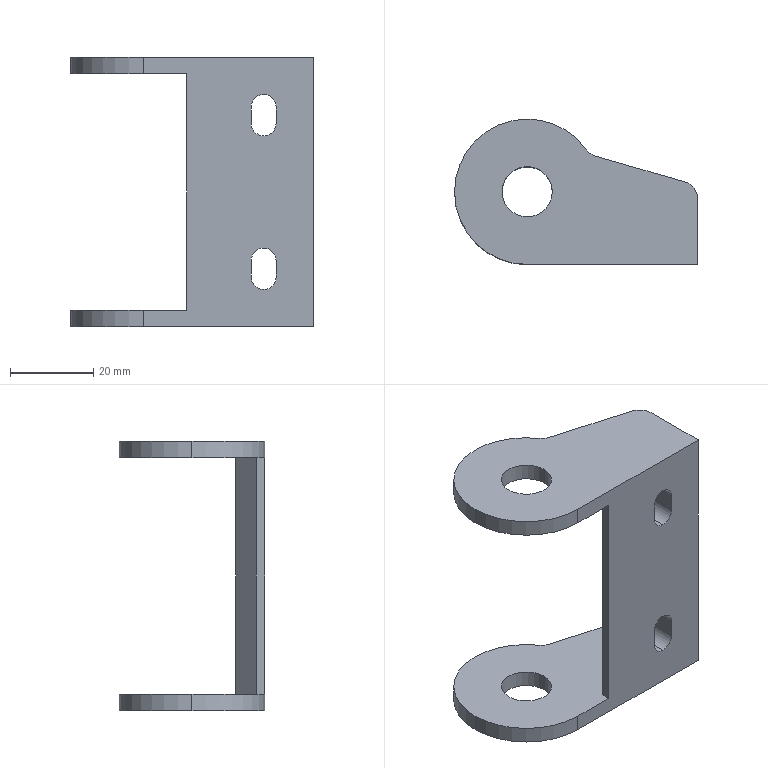Part | SolidWorks | features BaseBody 1 | 1 solid | 33 faces | box 58.5 x 35 x 65 mm | volume 22276 mm3 | cylinder 18 | plane 15 | commonest cylinder face diameters 6 x6 8 x4 12.1 x4 35 x4
STEP:
#1=CARTESIAN_POINT('',(-6.05,17.5,-28.5));
#2=VERTEX_POINT('',#1);
#3=CARTESIAN_POINT('',(6.05,17.5,-28.5));
#4=VERTEX_POINT('',#3);
#5=CARTESIAN_POINT('',(0.,17.5,-28.5));
#6=DIRECTION('',(0.,0.,1.));
#7=DIRECTION('',(1.,0.,0.));
#8=AXIS2_PLACEMENT_3D('',#5,#6,#7);
#9=CIRCLE('',#8,6.05);
#10=EDGE_CURVE('',#2,#4,#9,.T.);
#11=ORIENTED_EDGE('',*,*,#10,.T.);
#12=CARTESIAN_POINT('',(6.05,17.5,-32.5));
#13=VERTEX_POINT('',#12);
#14=CARTESIAN_POINT('',(6.05,17.5,32.5));
#15=DIRECTION('',(0.,0.,-1.));
#16=VECTOR('',#15,1000.);
#17=LINE('',#14,#16);
#18=EDGE_CURVE('',#4,#13,#17,.T.);
#19=ORIENTED_EDGE('',*,*,#18,.T.);
#20=CARTESIAN_POINT('',(-6.05,17.5,-32.5));
#21=VERTEX_POINT('',#20);
#22=CARTESIAN_POINT('',(0.,17.5,-32.5));
#23=DIRECTION('',(0.,0.,1.));
#24=DIRECTION('',(1.,0.,0.));
#25=AXIS2_PLACEMENT_3D('',#22,#23,#24);
#26=CIRCLE('',#25,6.05);
#27=EDGE_CURVE('',#21,#13,#26,.T.);
#28=ORIENTED_EDGE('',*,*,#27,.F.);
#29=CARTESIAN_POINT('',(-6.05,17.5,32.5));
#30=DIRECTION('',(0.,0.,-1.));
#31=VECTOR('',#30,1000.);
#32=LINE('',#29,#31);
#33=EDGE_CURVE('',#2,#21,#32,.T.);
#34=ORIENTED_EDGE('',*,*,#33,.F.);
#35=EDGE_LOOP('',(#11,#19,#28,#34));
#36=FACE_OUTER_BOUND('',#35,.T.);
#37=CARTESIAN_POINT('',(0.,17.5,32.5));
#38=DIRECTION('',(0.,0.,-1.));
#39=DIRECTION('',(-1.,0.,0.));
#40=AXIS2_PLACEMENT_3D('',#37,#38,#39);
#41=CYLINDRICAL_SURFACE('',#40,6.05);
#42=ADVANCED_FACE('',(#36),#41,.F.);
#43=CARTESIAN_POINT('',(-6.05,17.5,32.5));
#44=VERTEX_POINT('',#43);
#45=CARTESIAN_POINT('',(6.05,17.5,32.5));
#46=VERTEX_POINT('',#45);
#47=CARTESIAN_POINT('',(0.,17.5,32.5));
#48=DIRECTION('',(0.,0.,1.));
#49=DIRECTION('',(1.,0.,0.));
#50=AXIS2_PLACEMENT_3D('',#47,#48,#49);
#51=CIRCLE('',#50,6.05);
#52=EDGE_CURVE('',#44,#46,#51,.T.);
#53=ORIENTED_EDGE('',*,*,#52,.T.);
#54=CARTESIAN_POINT('',(6.05,17.5,28.5));
#55=VERTEX_POINT('',#54);
#56=CARTESIAN_POINT('',(6.05,17.5,32.5));
#57=DIRECTION('',(0.,0.,-1.));
#58=VECTOR('',#57,1000.);
#59=LINE('',#56,#58);
#60=EDGE_CURVE('',#46,#55,#59,.T.);
#61=ORIENTED_EDGE('',*,*,#60,.T.);
#62=CARTESIAN_POINT('',(-6.05,17.5,28.5));
#63=VERTEX_POINT('',#62);
#64=CARTESIAN_POINT('',(0.,17.5,28.5));
#65=DIRECTION('',(0.,0.,1.));
#66=DIRECTION('',(1.,0.,0.));
#67=AXIS2_PLACEMENT_3D('',#64,#65,#66);
#68=CIRCLE('',#67,6.05);
#69=EDGE_CURVE('',#63,#55,#68,.T.);
#70=ORIENTED_EDGE('',*,*,#69,.F.);
#71=CARTESIAN_POINT('',(-6.05,17.5,32.5));
#72=DIRECTION('',(0.,0.,-1.));
#73=VECTOR('',#72,1000.);
#74=LINE('',#71,#73);
#75=EDGE_CURVE('',#44,#63,#74,.T.);
#76=ORIENTED_EDGE('',*,*,#75,.F.);
#77=EDGE_LOOP('',(#53,#61,#70,#76));
#78=FACE_OUTER_BOUND('',#77,.T.);
#79=CARTESIAN_POINT('',(0.,17.5,32.5));
#80=DIRECTION('',(0.,0.,-1.));
#81=DIRECTION('',(-1.,0.,0.));
#82=AXIS2_PLACEMENT_3D('',#79,#80,#81);
#83=CYLINDRICAL_SURFACE('',#82,6.05);
#84=ADVANCED_FACE('',(#78),#83,.F.);
#85=CARTESIAN_POINT('',(29.,7.,13.5));
#86=VERTEX_POINT('',#85);
#87=CARTESIAN_POINT('',(32.,7.,16.5));
#88=VERTEX_POINT('',#87);
#89=CARTESIAN_POINT('',(29.,7.,16.5));
#90=DIRECTION('',(0.,-1.,0.));
#91=DIRECTION('',(-1.,0.,0.));
#92=AXIS2_PLACEMENT_3D('',#89,#90,#91);
#93=CIRCLE('',#92,3.);
#94=EDGE_CURVE('',#86,#88,#93,.T.);
#95=ORIENTED_EDGE('',*,*,#94,.F.);
#96=CARTESIAN_POINT('',(29.,0.,13.5));
#97=VERTEX_POINT('',#96);
#98=CARTESIAN_POINT('',(29.,10.,13.5));
#99=DIRECTION('',(0.,-1.,0.));
#100=VECTOR('',#99,1000.);
#101=LINE('',#98,#100);
#102=EDGE_CURVE('',#86,#97,#101,.T.);
#103=ORIENTED_EDGE('',*,*,#102,.T.);
#104=CARTESIAN_POINT('',(32.,0.,16.5));
#105=VERTEX_POINT('',#104);
#106=CARTESIAN_POINT('',(29.,0.,16.5));
#107=DIRECTION('',(0.,1.,0.));
#108=DIRECTION('',(1.,0.,0.));
#109=AXIS2_PLACEMENT_3D('',#106,#107,#108);
#110=CIRCLE('',#109,3.);
#111=EDGE_CURVE('',#105,#97,#110,.T.);
#112=ORIENTED_EDGE('',*,*,#111,.F.);
#113=CARTESIAN_POINT('',(32.,7.,16.5));
#114=DIRECTION('',(0.,-1.,0.));
#115=VECTOR('',#114,1000.);
#116=LINE('',#113,#115);
#117=EDGE_CURVE('',#88,#105,#116,.T.);
#118=ORIENTED_EDGE('',*,*,#117,.F.);
#119=EDGE_LOOP('',(#95,#103,#112,#118));
#120=FACE_OUTER_BOUND('',#119,.T.);
#121=CARTESIAN_POINT('',(29.,10.,16.5));
#122=DIRECTION('',(0.,-1.,0.));
#123=DIRECTION('',(0.,0.,-1.));
#124=AXIS2_PLACEMENT_3D('',#121,#122,#123);
#125=CYLINDRICAL_SURFACE('',#124,3.);
#126=ADVANCED_FACE('',(#120),#125,.F.);
#127=CARTESIAN_POINT('',(29.,7.,-23.5));
#128=VERTEX_POINT('',#127);
#129=CARTESIAN_POINT('',(32.,7.,-20.5));
#130=VERTEX_POINT('',#129);
#131=CARTESIAN_POINT('',(29.,7.,-20.5));
#132=DIRECTION('',(0.,-1.,0.));
#133=DIRECTION('',(-1.,0.,0.));
#134=AXIS2_PLACEMENT_3D('',#131,#132,#133);
#135=CIRCLE('',#134,3.);
#136=EDGE_CURVE('',#128,#130,#135,.T.);
#137=ORIENTED_EDGE('',*,*,#136,.F.);
#138=CARTESIAN_POINT('',(29.,0.,-23.5));
#139=VERTEX_POINT('',#138);
#140=CARTESIAN_POINT('',(29.,10.,-23.5));
#141=DIRECTION('',(0.,-1.,0.));
#142=VECTOR('',#141,1000.);
#143=LINE('',#140,#142);
#144=EDGE_CURVE('',#128,#139,#143,.T.);
#145=ORIENTED_EDGE('',*,*,#144,.T.);
#146=CARTESIAN_POINT('',(32.,0.,-20.5));
#147=VERTEX_POINT('',#146);
#148=CARTESIAN_POINT('',(29.,0.,-20.5));
#149=DIRECTION('',(0.,1.,0.));
#150=DIRECTION('',(1.,0.,0.));
#151=AXIS2_PLACEMENT_3D('',#148,#149,#150);
#152=CIRCLE('',#151,3.);
#153=EDGE_CURVE('',#147,#139,#152,.T.);
#154=ORIENTED_EDGE('',*,*,#153,.F.);
#155=CARTESIAN_POINT('',(32.,7.,-20.5));
#156=DIRECTION('',(0.,-1.,0.));
#157=VECTOR('',#156,1000.);
#158=LINE('',#155,#157);
#159=EDGE_CURVE('',#130,#147,#158,.T.);
#160=ORIENTED_EDGE('',*,*,#159,.F.);
#161=EDGE_LOOP('',(#137,#145,#154,#160));
#162=FACE_OUTER_BOUND('',#161,.T.);
#163=CARTESIAN_POINT('',(29.,10.,-20.5));
#164=DIRECTION('',(0.,-1.,0.));
#165=DIRECTION('',(0.,0.,-1.));
#166=AXIS2_PLACEMENT_3D('',#163,#164,#165);
#167=CYLINDRICAL_SURFACE('',#166,3.);
#168=ADVANCED_FACE('',(#162),#167,.F.);
#169=CARTESIAN_POINT('',(-17.5,17.5,-28.5));
#170=VERTEX_POINT('',#169);
#171=CARTESIAN_POINT('',(0.,0.,-28.5));
#172=VERTEX_POINT('',#171);
#173=CARTESIAN_POINT('',(0.,17.5,-28.5));
#174=DIRECTION('',(0.,0.,1.));
#175=DIRECTION('',(0.8159,0.5783,0.));
#176=AXIS2_PLACEMENT_3D('',#173,#174,#175);
#177=CIRCLE('',#176,17.5);
#178=EDGE_CURVE('',#170,#172,#177,.T.);
#179=ORIENTED_EDGE('',*,*,#178,.F.);
#180=CARTESIAN_POINT('',(-17.5,17.5,-32.5));
#181=VERTEX_POINT('',#180);
#182=CARTESIAN_POINT('',(-17.5,17.5,32.5));
#183=DIRECTION('',(0.,0.,-1.));
#184=VECTOR('',#183,1000.);
#185=LINE('',#182,#184);
#186=EDGE_CURVE('',#170,#181,#185,.T.);
#187=ORIENTED_EDGE('',*,*,#186,.T.);
#188=CARTESIAN_POINT('',(0.,0.,-32.5));
#189=VERTEX_POINT('',#188);
#190=CARTESIAN_POINT('',(0.,17.5,-32.5));
#191=DIRECTION('',(0.,0.,1.));
#192=DIRECTION('',(0.8159,0.5783,0.));
#193=AXIS2_PLACEMENT_3D('',#190,#191,#192);
#194=CIRCLE('',#193,17.5);
#195=EDGE_CURVE('',#181,#189,#194,.T.);
#196=ORIENTED_EDGE('',*,*,#195,.T.);
#197=CARTESIAN_POINT('',(0.,0.,-28.5));
#198=DIRECTION('',(0.,0.,-1.));
#199=VECTOR('',#198,1000.);
#200=LINE('',#197,#199);
#201=EDGE_CURVE('',#172,#189,#200,.T.);
#202=ORIENTED_EDGE('',*,*,#201,.F.);
#203=EDGE_LOOP('',(#179,#187,#196,#202));
#204=FACE_OUTER_BOUND('',#203,.T.);
#205=CARTESIAN_POINT('',(0.,17.5,32.5));
#206=DIRECTION('',(0.,0.,-1.));
#207=DIRECTION('',(-1.,0.,0.));
#208=AXIS2_PLACEMENT_3D('',#205,#206,#207);
#209=CYLINDRICAL_SURFACE('',#208,17.5);
#210=ADVANCED_FACE('',(#204),#209,.T.);
#211=CARTESIAN_POINT('',(-17.5,17.5,32.5));
#212=VERTEX_POINT('',#211);
#213=CARTESIAN_POINT('',(0.,0.,32.5));
#214=VERTEX_POINT('',#213);
#215=CARTESIAN_POINT('',(0.,17.5,32.5));
#216=DIRECTION('',(0.,0.,1.));
#217=DIRECTION('',(0.8159,0.5783,0.));
#218=AXIS2_PLACEMENT_3D('',#215,#216,#217);
#219=CIRCLE('',#218,17.5);
#220=EDGE_CURVE('',#212,#214,#219,.T.);
#221=ORIENTED_EDGE('',*,*,#220,.F.);
#222=CARTESIAN_POINT('',(-17.5,17.5,28.5));
#223=VERTEX_POINT('',#222);
#224=CARTESIAN_POINT('',(-17.5,17.5,32.5));
#225=DIRECTION('',(0.,0.,-1.));
#226=VECTOR('',#225,1000.);
#227=LINE('',#224,#226);
#228=EDGE_CURVE('',#212,#223,#227,.T.);
#229=ORIENTED_EDGE('',*,*,#228,.T.);
#230=CARTESIAN_POINT('',(0.,0.,28.5));
#231=VERTEX_POINT('',#230);
#232=CARTESIAN_POINT('',(0.,17.5,28.5));
#233=DIRECTION('',(0.,0.,1.));
#234=DIRECTION('',(0.8159,0.5783,0.));
#235=AXIS2_PLACEMENT_3D('',#232,#233,#234);
#236=CIRCLE('',#235,17.5);
#237=EDGE_CURVE('',#223,#231,#236,.T.);
#238=ORIENTED_EDGE('',*,*,#237,.T.);
#239=CARTESIAN_POINT('',(0.,0.,32.5));
#240=DIRECTION('',(0.,0.,-1.));
#241=VECTOR('',#240,1000.);
#242=LINE('',#239,#241);
#243=EDGE_CURVE('',#214,#231,#242,.T.);
#244=ORIENTED_EDGE('',*,*,#243,.F.);
#245=EDGE_LOOP('',(#221,#229,#238,#244));
#246=FACE_OUTER_BOUND('',#245,.T.);
#247=CARTESIAN_POINT('',(0.,17.5,32.5));
#248=DIRECTION('',(0.,0.,-1.));
#249=DIRECTION('',(-1.,0.,0.));
#250=AXIS2_PLACEMENT_3D('',#247,#248,#249);
#251=CYLINDRICAL_SURFACE('',#250,17.5);
#252=ADVANCED_FACE('',(#246),#251,.T.);
#253=ORIENTED_EDGE('',*,*,#243,.T.);
#254=CARTESIAN_POINT('',(10.5,0.,28.5));
#255=VERTEX_POINT('',#254);
#256=CARTESIAN_POINT('',(0.,0.,28.5));
#257=DIRECTION('',(1.,0.,0.));
#258=VECTOR('',#257,1000.);
#259=LINE('',#256,#258);
#260=EDGE_CURVE('',#231,#255,#259,.T.);
#261=ORIENTED_EDGE('',*,*,#260,.T.);
#262=CARTESIAN_POINT('',(10.5,0.,-28.5));
#263=VERTEX_POINT('',#262);
#264=CARTESIAN_POINT('',(10.5,0.,28.5));
#265=DIRECTION('',(0.,0.,-1.));
#266=VECTOR('',#265,1000.);
#267=LINE('',#264,#266);
#268=EDGE_CURVE('',#255,#263,#267,.T.);
#269=ORIENTED_EDGE('',*,*,#268,.T.);
#270=CARTESIAN_POINT('',(0.,0.,-28.5));
#271=DIRECTION('',(1.,0.,0.));
#272=VECTOR('',#271,1000.);
#273=LINE('',#270,#272);
#274=EDGE_CURVE('',#172,#263,#273,.T.);
#275=ORIENTED_EDGE('',*,*,#274,.F.);
#276=ORIENTED_EDGE('',*,*,#201,.T.);
#277=CARTESIAN_POINT('',(41.,0.,-32.5));
#278=VERTEX_POINT('',#277);
#279=CARTESIAN_POINT('',(0.,0.,-32.5));
#280=DIRECTION('',(1.,0.,0.));
#281=VECTOR('',#280,1000.);
#282=LINE('',#279,#281);
#283=EDGE_CURVE('',#189,#278,#282,.T.);
#284=ORIENTED_EDGE('',*,*,#283,.T.);
#285=CARTESIAN_POINT('',(41.,0.,32.5));
#286=VERTEX_POINT('',#285);
#287=CARTESIAN_POINT('',(41.,0.,32.5));
#288=DIRECTION('',(0.,0.,-1.));
#289=VECTOR('',#288,1000.);
#290=LINE('',#287,#289);
#291=EDGE_CURVE('',#286,#278,#290,.T.);
#292=ORIENTED_EDGE('',*,*,#291,.F.);
#293=CARTESIAN_POINT('',(0.,0.,32.5));
#294=DIRECTION('',(1.,0.,0.));
#295=VECTOR('',#294,1000.);
#296=LINE('',#293,#295);
#297=EDGE_CURVE('',#214,#286,#296,.T.);
#298=ORIENTED_EDGE('',*,*,#297,.F.);
#299=EDGE_LOOP('',(#253,#261,#269,#275,#276,#284,#292,#298));
#300=FACE_OUTER_BOUND('',#299,.T.);
#301=CARTESIAN_POINT('',(26.,0.,-20.5));
#302=VERTEX_POINT('',#301);
#303=CARTESIAN_POINT('',(26.,0.,-16.5));
#304=VERTEX_POINT('',#303);
#305=CARTESIAN_POINT('',(26.,0.,-20.5));
#306=DIRECTION('',(0.,0.,1.));
#307=VECTOR('',#306,1000.);
#308=LINE('',#305,#307);
#309=EDGE_CURVE('',#302,#304,#308,.T.);
#310=ORIENTED_EDGE('',*,*,#309,.T.);
#311=CARTESIAN_POINT('',(32.,0.,-16.5));
#312=VERTEX_POINT('',#311);
#313=CARTESIAN_POINT('',(29.,0.,-16.5));
#314=DIRECTION('',(0.,1.,0.));
#315=DIRECTION('',(-1.,0.,0.));
#316=AXIS2_PLACEMENT_3D('',#313,#314,#315);
#317=CIRCLE('',#316,3.);
#318=EDGE_CURVE('',#304,#312,#317,.T.);
#319=ORIENTED_EDGE('',*,*,#318,.T.);
#320=CARTESIAN_POINT('',(32.,0.,-16.5));
#321=DIRECTION('',(0.,0.,-1.));
#322=VECTOR('',#321,1000.);
#323=LINE('',#320,#322);
#324=EDGE_CURVE('',#312,#147,#323,.T.);
#325=ORIENTED_EDGE('',*,*,#324,.T.);
#326=ORIENTED_EDGE('',*,*,#153,.T.);
#327=CARTESIAN_POINT('',(29.,0.,-20.5));
#328=DIRECTION('',(0.,1.,0.));
#329=DIRECTION('',(1.,0.,0.));
#330=AXIS2_PLACEMENT_3D('',#327,#328,#329);
#331=CIRCLE('',#330,3.);
#332=EDGE_CURVE('',#139,#302,#331,.T.);
#333=ORIENTED_EDGE('',*,*,#332,.T.);
#334=EDGE_LOOP('',(#310,#319,#325,#326,#333));
#335=FACE_BOUND('',#334,.T.);
#336=ORIENTED_EDGE('',*,*,#111,.T.);
#337=CARTESIAN_POINT('',(26.,0.,16.5));
#338=VERTEX_POINT('',#337);
#339=CARTESIAN_POINT('',(29.,0.,16.5));
#340=DIRECTION('',(0.,1.,0.));
#341=DIRECTION('',(1.,0.,0.));
#342=AXIS2_PLACEMENT_3D('',#339,#340,#341);
#343=CIRCLE('',#342,3.);
#344=EDGE_CURVE('',#97,#338,#343,.T.);
#345=ORIENTED_EDGE('',*,*,#344,.T.);
#346=CARTESIAN_POINT('',(26.,0.,20.5));
#347=VERTEX_POINT('',#346);
#348=CARTESIAN_POINT('',(26.,0.,16.5));
#349=DIRECTION('',(0.,0.,1.));
#350=VECTOR('',#349,1000.);
#351=LINE('',#348,#350);
#352=EDGE_CURVE('',#338,#347,#351,.T.);
#353=ORIENTED_EDGE('',*,*,#352,.T.);
#354=CARTESIAN_POINT('',(32.,0.,20.5));
#355=VERTEX_POINT('',#354);
#356=CARTESIAN_POINT('',(29.,0.,20.5));
#357=DIRECTION('',(0.,1.,0.));
#358=DIRECTION('',(-1.,0.,0.));
#359=AXIS2_PLACEMENT_3D('',#356,#357,#358);
#360=CIRCLE('',#359,3.);
#361=EDGE_CURVE('',#347,#355,#360,.T.);
#362=ORIENTED_EDGE('',*,*,#361,.T.);
#363=CARTESIAN_POINT('',(32.,0.,20.5));
#364=DIRECTION('',(0.,0.,-1.));
#365=VECTOR('',#364,1000.);
#366=LINE('',#363,#365);
#367=EDGE_CURVE('',#355,#105,#366,.T.);
#368=ORIENTED_EDGE('',*,*,#367,.T.);
#369=EDGE_LOOP('',(#336,#345,#353,#362,#368));
#370=FACE_BOUND('',#369,.T.);
#371=CARTESIAN_POINT('',(0.,0.,32.5));
#372=DIRECTION('',(0.,1.,0.));
#373=DIRECTION('',(0.,0.,1.));
#374=AXIS2_PLACEMENT_3D('',#371,#372,#373);
#375=PLANE('',#374);
#376=ADVANCED_FACE('',(#300,#335,#370),#375,.F.);
#377=ORIENTED_EDGE('',*,*,#228,.F.);
#378=CARTESIAN_POINT('',(14.278,27.619,32.5));
#379=VERTEX_POINT('',#378);
#380=CARTESIAN_POINT('',(0.,17.5,32.5));
#381=DIRECTION('',(0.,0.,1.));
#382=DIRECTION('',(0.8159,0.5783,0.));
#383=AXIS2_PLACEMENT_3D('',#380,#381,#382);
#384=CIRCLE('',#383,17.5);
#385=EDGE_CURVE('',#379,#212,#384,.T.);
#386=ORIENTED_EDGE('',*,*,#385,.F.);
#387=CARTESIAN_POINT('',(14.278,27.619,28.5));
#388=VERTEX_POINT('',#387);
#389=CARTESIAN_POINT('',(14.278,27.619,32.5));
#390=DIRECTION('',(0.,0.,-1.));
#391=VECTOR('',#390,1000.);
#392=LINE('',#389,#391);
#393=EDGE_CURVE('',#379,#388,#392,.T.);
#394=ORIENTED_EDGE('',*,*,#393,.T.);
#395=CARTESIAN_POINT('',(0.,17.5,28.5));
#396=DIRECTION('',(0.,0.,1.));
#397=DIRECTION('',(0.8159,0.5783,0.));
#398=AXIS2_PLACEMENT_3D('',#395,#396,#397);
#399=CIRCLE('',#398,17.5);
#400=EDGE_CURVE('',#388,#223,#399,.T.);
#401=ORIENTED_EDGE('',*,*,#400,.T.);
#402=EDGE_LOOP('',(#377,#386,#394,#401));
#403=FACE_OUTER_BOUND('',#402,.T.);
#404=CARTESIAN_POINT('',(0.,17.5,32.5));
#405=DIRECTION('',(0.,0.,-1.));
#406=DIRECTION('',(-1.,0.,0.));
#407=AXIS2_PLACEMENT_3D('',#404,#405,#406);
#408=CYLINDRICAL_SURFACE('',#407,17.5);
#409=ADVANCED_FACE('',(#403),#408,.T.);
#410=ORIENTED_EDGE('',*,*,#69,.T.);
#411=CARTESIAN_POINT('',(0.,17.5,28.5));
#412=DIRECTION('',(0.,0.,1.));
#413=DIRECTION('',(1.,0.,0.));
#414=AXIS2_PLACEMENT_3D('',#411,#412,#413);
#415=CIRCLE('',#414,6.05);
#416=EDGE_CURVE('',#55,#63,#415,.T.);
#417=ORIENTED_EDGE('',*,*,#416,.T.);
#418=EDGE_LOOP('',(#410,#417));
#419=FACE_BOUND('',#418,.T.);
#420=CARTESIAN_POINT('',(41.,7.,28.5));
#421=VERTEX_POINT('',#420);
#422=CARTESIAN_POINT('',(41.,15.991,28.5));
#423=VERTEX_POINT('',#422);
#424=CARTESIAN_POINT('',(41.,7.,28.5));
#425=DIRECTION('',(0.,1.,0.));
#426=VECTOR('',#425,1000.);
#427=LINE('',#424,#426);
#428=EDGE_CURVE('',#421,#423,#427,.T.);
#429=ORIENTED_EDGE('',*,*,#428,.F.);
#430=CARTESIAN_POINT('',(15.5,7.,28.5));
#431=VERTEX_POINT('',#430);
#432=CARTESIAN_POINT('',(15.5,7.,28.5));
#433=DIRECTION('',(1.,0.,0.));
#434=VECTOR('',#433,1000.);
#435=LINE('',#432,#434);
#436=EDGE_CURVE('',#431,#421,#435,.T.);
#437=ORIENTED_EDGE('',*,*,#436,.F.);
#438=CARTESIAN_POINT('',(10.5,2.,28.5));
#439=VERTEX_POINT('',#438);
#440=CARTESIAN_POINT('',(10.5,2.,28.5));
#441=DIRECTION('',(0.7071,0.7071,0.));
#442=VECTOR('',#441,1000.);
#443=LINE('',#440,#442);
#444=EDGE_CURVE('',#439,#431,#443,.T.);
#445=ORIENTED_EDGE('',*,*,#444,.F.);
#446=CARTESIAN_POINT('',(10.5,0.,28.5));
#447=DIRECTION('',(0.,1.,0.));
#448=VECTOR('',#447,1000.);
#449=LINE('',#446,#448);
#450=EDGE_CURVE('',#255,#439,#449,.T.);
#451=ORIENTED_EDGE('',*,*,#450,.F.);
#452=ORIENTED_EDGE('',*,*,#260,.F.);
#453=ORIENTED_EDGE('',*,*,#237,.F.);
#454=ORIENTED_EDGE('',*,*,#400,.F.);
#455=CARTESIAN_POINT('',(16.432,26.089,28.5));
#456=VERTEX_POINT('',#455);
#457=CARTESIAN_POINT('',(17.541,29.932,28.5));
#458=DIRECTION('',(0.,0.,1.));
#459=DIRECTION('',(-0.8159,-0.5783,0.));
#460=AXIS2_PLACEMENT_3D('',#457,#458,#459);
#461=CIRCLE('',#460,4.);
#462=EDGE_CURVE('',#388,#456,#461,.T.);
#463=ORIENTED_EDGE('',*,*,#462,.T.);
#464=CARTESIAN_POINT('',(38.109,19.834,28.5));
#465=VERTEX_POINT('',#464);
#466=CARTESIAN_POINT('',(38.109,19.834,28.5));
#467=DIRECTION('',(-0.9608,0.2772,0.));
#468=VECTOR('',#467,1000.);
#469=LINE('',#466,#468);
#470=EDGE_CURVE('',#465,#456,#469,.T.);
#471=ORIENTED_EDGE('',*,*,#470,.F.);
#472=CARTESIAN_POINT('',(37.,15.991,28.5));
#473=DIRECTION('',(0.,0.,1.));
#474=DIRECTION('',(1.,0.,0.));
#475=AXIS2_PLACEMENT_3D('',#472,#473,#474);
#476=CIRCLE('',#475,4.);
#477=EDGE_CURVE('',#423,#465,#476,.T.);
#478=ORIENTED_EDGE('',*,*,#477,.F.);
#479=EDGE_LOOP('',(#429,#437,#445,#451,#452,#453,#454,#463,#471,#478));
#480=FACE_OUTER_BOUND('',#479,.T.);
#481=CARTESIAN_POINT('',(0.,0.,28.5));
#482=DIRECTION('',(0.,0.,1.));
#483=DIRECTION('',(1.,0.,0.));
#484=AXIS2_PLACEMENT_3D('',#481,#482,#483);
#485=PLANE('',#484);
#486=ADVANCED_FACE('',(#419,#480),#485,.F.);
#487=CARTESIAN_POINT('',(10.5,2.,-28.5));
#488=VERTEX_POINT('',#487);
#489=CARTESIAN_POINT('',(10.5,0.,-28.5));
#490=DIRECTION('',(0.,1.,0.));
#491=VECTOR('',#490,1000.);
#492=LINE('',#489,#491);
#493=EDGE_CURVE('',#263,#488,#492,.T.);
#494=ORIENTED_EDGE('',*,*,#493,.F.);
#495=ORIENTED_EDGE('',*,*,#268,.F.);
#496=ORIENTED_EDGE('',*,*,#450,.T.);
#497=CARTESIAN_POINT('',(10.5,2.,28.5));
#498=DIRECTION('',(0.,0.,-1.));
#499=VECTOR('',#498,1000.);
#500=LINE('',#497,#499);
#501=EDGE_CURVE('',#439,#488,#500,.T.);
#502=ORIENTED_EDGE('',*,*,#501,.T.);
#503=EDGE_LOOP('',(#494,#495,#496,#502));
#504=FACE_OUTER_BOUND('',#503,.T.);
#505=CARTESIAN_POINT('',(10.5,0.,28.5));
#506=DIRECTION('',(-1.,0.,0.));
#507=DIRECTION('',(0.,0.,1.));
#508=AXIS2_PLACEMENT_3D('',#505,#506,#507);
#509=PLANE('',#508);
#510=ADVANCED_FACE('',(#504),#509,.T.);
#511=ORIENTED_EDGE('',*,*,#10,.F.);
#512=CARTESIAN_POINT('',(0.,17.5,-28.5));
#513=DIRECTION('',(0.,0.,1.));
#514=DIRECTION('',(1.,0.,0.));
#515=AXIS2_PLACEMENT_3D('',#512,#513,#514);
#516=CIRCLE('',#515,6.05);
#517=EDGE_CURVE('',#4,#2,#516,.T.);
#518=ORIENTED_EDGE('',*,*,#517,.F.);
#519=EDGE_LOOP('',(#511,#518));
#520=FACE_BOUND('',#519,.T.);
#521=CARTESIAN_POINT('',(41.,15.991,-28.5));
#522=VERTEX_POINT('',#521);
#523=CARTESIAN_POINT('',(38.109,19.834,-28.5));
#524=VERTEX_POINT('',#523);
#525=CARTESIAN_POINT('',(37.,15.991,-28.5));
#526=DIRECTION('',(0.,0.,1.));
#527=DIRECTION('',(1.,0.,0.));
#528=AXIS2_PLACEMENT_3D('',#525,#526,#527);
#529=CIRCLE('',#528,4.);
#530=EDGE_CURVE('',#522,#524,#529,.T.);
#531=ORIENTED_EDGE('',*,*,#530,.T.);
#532=CARTESIAN_POINT('',(16.432,26.089,-28.5));
#533=VERTEX_POINT('',#532);
#534=CARTESIAN_POINT('',(38.109,19.834,-28.5));
#535=DIRECTION('',(-0.9608,0.2772,0.));
#536=VECTOR('',#535,1000.);
#537=LINE('',#534,#536);
#538=EDGE_CURVE('',#524,#533,#537,.T.);
#539=ORIENTED_EDGE('',*,*,#538,.T.);
#540=CARTESIAN_POINT('',(14.278,27.619,-28.5));
#541=VERTEX_POINT('',#540);
#542=CARTESIAN_POINT('',(17.541,29.932,-28.5));
#543=DIRECTION('',(0.,0.,1.));
#544=DIRECTION('',(-0.8159,-0.5783,0.));
#545=AXIS2_PLACEMENT_3D('',#542,#543,#544);
#546=CIRCLE('',#545,4.);
#547=EDGE_CURVE('',#541,#533,#546,.T.);
#548=ORIENTED_EDGE('',*,*,#547,.F.);
#549=CARTESIAN_POINT('',(0.,17.5,-28.5));
#550=DIRECTION('',(0.,0.,1.));
#551=DIRECTION('',(0.8159,0.5783,0.));
#552=AXIS2_PLACEMENT_3D('',#549,#550,#551);
#553=CIRCLE('',#552,17.5);
#554=EDGE_CURVE('',#541,#170,#553,.T.);
#555=ORIENTED_EDGE('',*,*,#554,.T.);
#556=ORIENTED_EDGE('',*,*,#178,.T.);
#557=ORIENTED_EDGE('',*,*,#274,.T.);
#558=ORIENTED_EDGE('',*,*,#493,.T.);
#559=CARTESIAN_POINT('',(15.5,7.,-28.5));
#560=VERTEX_POINT('',#559);
#561=CARTESIAN_POINT('',(10.5,2.,-28.5));
#562=DIRECTION('',(0.7071,0.7071,0.));
#563=VECTOR('',#562,1000.);
#564=LINE('',#561,#563);
#565=EDGE_CURVE('',#488,#560,#564,.T.);
#566=ORIENTED_EDGE('',*,*,#565,.T.);
#567=CARTESIAN_POINT('',(41.,7.,-28.5));
#568=VERTEX_POINT('',#567);
#569=CARTESIAN_POINT('',(15.5,7.,-28.5));
#570=DIRECTION('',(1.,0.,0.));
#571=VECTOR('',#570,1000.);
#572=LINE('',#569,#571);
#573=EDGE_CURVE('',#560,#568,#572,.T.);
#574=ORIENTED_EDGE('',*,*,#573,.T.);
#575=CARTESIAN_POINT('',(41.,7.,-28.5));
#576=DIRECTION('',(0.,1.,0.));
#577=VECTOR('',#576,1000.);
#578=LINE('',#575,#577);
#579=EDGE_CURVE('',#568,#522,#578,.T.);
#580=ORIENTED_EDGE('',*,*,#579,.T.);
#581=EDGE_LOOP('',(#531,#539,#548,#555,#556,#557,#558,#566,#574,#580));
#582=FACE_OUTER_BOUND('',#581,.T.);
#583=CARTESIAN_POINT('',(0.,0.,-28.5));
#584=DIRECTION('',(0.,0.,1.));
#585=DIRECTION('',(1.,0.,0.));
#586=AXIS2_PLACEMENT_3D('',#583,#584,#585);
#587=PLANE('',#586);
#588=ADVANCED_FACE('',(#520,#582),#587,.T.);
#589=ORIENTED_EDGE('',*,*,#186,.F.);
#590=ORIENTED_EDGE('',*,*,#554,.F.);
#591=CARTESIAN_POINT('',(14.278,27.619,-32.5));
#592=VERTEX_POINT('',#591);
#593=CARTESIAN_POINT('',(14.278,27.619,-28.5));
#594=DIRECTION('',(0.,0.,-1.));
#595=VECTOR('',#594,1000.);
#596=LINE('',#593,#595);
#597=EDGE_CURVE('',#541,#592,#596,.T.);
#598=ORIENTED_EDGE('',*,*,#597,.T.);
#599=CARTESIAN_POINT('',(0.,17.5,-32.5));
#600=DIRECTION('',(0.,0.,1.));
#601=DIRECTION('',(0.8159,0.5783,0.));
#602=AXIS2_PLACEMENT_3D('',#599,#600,#601);
#603=CIRCLE('',#602,17.5);
#604=EDGE_CURVE('',#592,#181,#603,.T.);
#605=ORIENTED_EDGE('',*,*,#604,.T.);
#606=EDGE_LOOP('',(#589,#590,#598,#605));
#607=FACE_OUTER_BOUND('',#606,.T.);
#608=CARTESIAN_POINT('',(0.,17.5,32.5));
#609=DIRECTION('',(0.,0.,-1.));
#610=DIRECTION('',(-1.,0.,0.));
#611=AXIS2_PLACEMENT_3D('',#608,#609,#610);
#612=CYLINDRICAL_SURFACE('',#611,17.5);
#613=ADVANCED_FACE('',(#607),#612,.T.);
#614=CARTESIAN_POINT('',(16.432,26.089,-32.5));
#615=VERTEX_POINT('',#614);
#616=CARTESIAN_POINT('',(17.541,29.932,-32.5));
#617=DIRECTION('',(0.,0.,1.));
#618=DIRECTION('',(-0.8159,-0.5783,0.));
#619=AXIS2_PLACEMENT_3D('',#616,#617,#618);
#620=CIRCLE('',#619,4.);
#621=EDGE_CURVE('',#592,#615,#620,.T.);
#622=ORIENTED_EDGE('',*,*,#621,.T.);
#623=CARTESIAN_POINT('',(38.109,19.834,-32.5));
#624=VERTEX_POINT('',#623);
#625=CARTESIAN_POINT('',(38.109,19.834,-32.5));
#626=DIRECTION('',(-0.9608,0.2772,0.));
#627=VECTOR('',#626,1000.);
#628=LINE('',#625,#627);
#629=EDGE_CURVE('',#624,#615,#628,.T.);
#630=ORIENTED_EDGE('',*,*,#629,.F.);
#631=CARTESIAN_POINT('',(41.,15.991,-32.5));
#632=VERTEX_POINT('',#631);
#633=CARTESIAN_POINT('',(37.,15.991,-32.5));
#634=DIRECTION('',(0.,0.,1.));
#635=DIRECTION('',(1.,0.,0.));
#636=AXIS2_PLACEMENT_3D('',#633,#634,#635);
#637=CIRCLE('',#636,4.);
#638=EDGE_CURVE('',#632,#624,#637,.T.);
#639=ORIENTED_EDGE('',*,*,#638,.F.);
#640=CARTESIAN_POINT('',(41.,0.,-32.5));
#641=DIRECTION('',(0.,1.,0.));
#642=VECTOR('',#641,1000.);
#643=LINE('',#640,#642);
#644=EDGE_CURVE('',#278,#632,#643,.T.);
#645=ORIENTED_EDGE('',*,*,#644,.F.);
#646=ORIENTED_EDGE('',*,*,#283,.F.);
#647=ORIENTED_EDGE('',*,*,#195,.F.);
#648=ORIENTED_EDGE('',*,*,#604,.F.);
#649=EDGE_LOOP('',(#622,#630,#639,#645,#646,#647,#648));
#650=FACE_OUTER_BOUND('',#649,.T.);
#651=ORIENTED_EDGE('',*,*,#27,.T.);
#652=CARTESIAN_POINT('',(0.,17.5,-32.5));
#653=DIRECTION('',(0.,0.,1.));
#654=DIRECTION('',(1.,0.,0.));
#655=AXIS2_PLACEMENT_3D('',#652,#653,#654);
#656=CIRCLE('',#655,6.05);
#657=EDGE_CURVE('',#13,#21,#656,.T.);
#658=ORIENTED_EDGE('',*,*,#657,.T.);
#659=EDGE_LOOP('',(#651,#658));
#660=FACE_BOUND('',#659,.T.);
#661=CARTESIAN_POINT('',(17.541,29.932,-32.5));
#662=DIRECTION('',(0.,0.,1.));
#663=DIRECTION('',(1.,0.,0.));
#664=AXIS2_PLACEMENT_3D('',#661,#662,#663);
#665=PLANE('',#664);
#666=ADVANCED_FACE('',(#650,#660),#665,.F.);
#667=CARTESIAN_POINT('',(41.,7.,28.5));
#668=DIRECTION('',(0.,0.,-1.));
#669=VECTOR('',#668,1000.);
#670=LINE('',#667,#669);
#671=EDGE_CURVE('',#421,#568,#670,.T.);
#672=ORIENTED_EDGE('',*,*,#671,.F.);
#673=ORIENTED_EDGE('',*,*,#428,.T.);
#674=CARTESIAN_POINT('',(41.,15.991,32.5));
#675=VERTEX_POINT('',#674);
#676=CARTESIAN_POINT('',(41.,15.991,32.5));
#677=DIRECTION('',(0.,0.,-1.));
#678=VECTOR('',#677,1000.);
#679=LINE('',#676,#678);
#680=EDGE_CURVE('',#675,#423,#679,.T.);
#681=ORIENTED_EDGE('',*,*,#680,.F.);
#682=CARTESIAN_POINT('',(41.,0.,32.5));
#683=DIRECTION('',(0.,1.,0.));
#684=VECTOR('',#683,1000.);
#685=LINE('',#682,#684);
#686=EDGE_CURVE('',#286,#675,#685,.T.);
#687=ORIENTED_EDGE('',*,*,#686,.F.);
#688=ORIENTED_EDGE('',*,*,#291,.T.);
#689=ORIENTED_EDGE('',*,*,#644,.T.);
#690=CARTESIAN_POINT('',(41.,15.991,-28.5));
#691=DIRECTION('',(0.,0.,-1.));
#692=VECTOR('',#691,1000.);
#693=LINE('',#690,#692);
#694=EDGE_CURVE('',#522,#632,#693,.T.);
#695=ORIENTED_EDGE('',*,*,#694,.F.);
#696=ORIENTED_EDGE('',*,*,#579,.F.);
#697=EDGE_LOOP('',(#672,#673,#681,#687,#688,#689,#695,#696));
#698=FACE_OUTER_BOUND('',#697,.T.);
#699=CARTESIAN_POINT('',(41.,0.,32.5));
#700=DIRECTION('',(-1.,0.,0.));
#701=DIRECTION('',(0.,0.,1.));
#702=AXIS2_PLACEMENT_3D('',#699,#700,#701);
#703=PLANE('',#702);
#704=ADVANCED_FACE('',(#698),#703,.F.);
#705=CARTESIAN_POINT('',(16.432,26.089,32.5));
#706=VERTEX_POINT('',#705);
#707=CARTESIAN_POINT('',(17.541,29.932,32.5));
#708=DIRECTION('',(0.,0.,1.));
#709=DIRECTION('',(-0.8159,-0.5783,0.));
#710=AXIS2_PLACEMENT_3D('',#707,#708,#709);
#711=CIRCLE('',#710,4.);
#712=EDGE_CURVE('',#379,#706,#711,.T.);
#713=ORIENTED_EDGE('',*,*,#712,.F.);
#714=ORIENTED_EDGE('',*,*,#385,.T.);
#715=ORIENTED_EDGE('',*,*,#220,.T.);
#716=ORIENTED_EDGE('',*,*,#297,.T.);
#717=ORIENTED_EDGE('',*,*,#686,.T.);
#718=CARTESIAN_POINT('',(38.109,19.834,32.5));
#719=VERTEX_POINT('',#718);
#720=CARTESIAN_POINT('',(37.,15.991,32.5));
#721=DIRECTION('',(0.,0.,1.));
#722=DIRECTION('',(1.,0.,0.));
#723=AXIS2_PLACEMENT_3D('',#720,#721,#722);
#724=CIRCLE('',#723,4.);
#725=EDGE_CURVE('',#675,#719,#724,.T.);
#726=ORIENTED_EDGE('',*,*,#725,.T.);
#727=CARTESIAN_POINT('',(38.109,19.834,32.5));
#728=DIRECTION('',(-0.9608,0.2772,0.));
#729=VECTOR('',#728,1000.);
#730=LINE('',#727,#729);
#731=EDGE_CURVE('',#719,#706,#730,.T.);
#732=ORIENTED_EDGE('',*,*,#731,.T.);
#733=EDGE_LOOP('',(#713,#714,#715,#716,#717,#726,#732));
#734=FACE_OUTER_BOUND('',#733,.T.);
#735=ORIENTED_EDGE('',*,*,#52,.F.);
#736=CARTESIAN_POINT('',(0.,17.5,32.5));
#737=DIRECTION('',(0.,0.,1.));
#738=DIRECTION('',(1.,0.,0.));
#739=AXIS2_PLACEMENT_3D('',#736,#737,#738);
#740=CIRCLE('',#739,6.05);
#741=EDGE_CURVE('',#46,#44,#740,.T.);
#742=ORIENTED_EDGE('',*,*,#741,.F.);
#743=EDGE_LOOP('',(#735,#742));
#744=FACE_BOUND('',#743,.T.);
#745=CARTESIAN_POINT('',(17.541,29.932,32.5));
#746=DIRECTION('',(0.,0.,1.));
#747=DIRECTION('',(1.,0.,0.));
#748=AXIS2_PLACEMENT_3D('',#745,#746,#747);
#749=PLANE('',#748);
#750=ADVANCED_FACE('',(#734,#744),#749,.T.);
#751=CARTESIAN_POINT('',(26.,7.,-16.5));
#752=VERTEX_POINT('',#751);
#753=CARTESIAN_POINT('',(26.,7.,-16.5));
#754=DIRECTION('',(0.,-1.,0.));
#755=VECTOR('',#754,1000.);
#756=LINE('',#753,#755);
#757=EDGE_CURVE('',#752,#304,#756,.T.);
#758=ORIENTED_EDGE('',*,*,#757,.T.);
#759=ORIENTED_EDGE('',*,*,#309,.F.);
#760=CARTESIAN_POINT('',(26.,7.,-20.5));
#761=VERTEX_POINT('',#760);
#762=CARTESIAN_POINT('',(26.,7.,-20.5));
#763=DIRECTION('',(0.,-1.,0.));
#764=VECTOR('',#763,1000.);
#765=LINE('',#762,#764);
#766=EDGE_CURVE('',#761,#302,#765,.T.);
#767=ORIENTED_EDGE('',*,*,#766,.F.);
#768=CARTESIAN_POINT('',(26.,7.,-16.5));
#769=DIRECTION('',(0.,0.,-1.));
#770=VECTOR('',#769,1000.);
#771=LINE('',#768,#770);
#772=EDGE_CURVE('',#752,#761,#771,.T.);
#773=ORIENTED_EDGE('',*,*,#772,.F.);
#774=EDGE_LOOP('',(#758,#759,#767,#773));
#775=FACE_OUTER_BOUND('',#774,.T.);
#776=CARTESIAN_POINT('',(26.,10.,-20.5));
#777=DIRECTION('',(1.,0.,0.));
#778=DIRECTION('',(0.,0.,-1.));
#779=AXIS2_PLACEMENT_3D('',#776,#777,#778);
#780=PLANE('',#779);
#781=ADVANCED_FACE('',(#775),#780,.T.);
#782=CARTESIAN_POINT('',(32.,7.,-16.5));
#783=VERTEX_POINT('',#782);
#784=CARTESIAN_POINT('',(32.,7.,-16.5));
#785=DIRECTION('',(0.,-1.,0.));
#786=VECTOR('',#785,1000.);
#787=LINE('',#784,#786);
#788=EDGE_CURVE('',#783,#312,#787,.T.);
#789=ORIENTED_EDGE('',*,*,#788,.T.);
#790=ORIENTED_EDGE('',*,*,#318,.F.);
#791=ORIENTED_EDGE('',*,*,#757,.F.);
#792=CARTESIAN_POINT('',(29.,7.,-16.5));
#793=DIRECTION('',(0.,-1.,0.));
#794=DIRECTION('',(1.,0.,0.));
#795=AXIS2_PLACEMENT_3D('',#792,#793,#794);
#796=CIRCLE('',#795,3.);
#797=EDGE_CURVE('',#783,#752,#796,.T.);
#798=ORIENTED_EDGE('',*,*,#797,.F.);
#799=EDGE_LOOP('',(#789,#790,#791,#798));
#800=FACE_OUTER_BOUND('',#799,.T.);
#801=CARTESIAN_POINT('',(29.,10.,-16.5));
#802=DIRECTION('',(0.,-1.,0.));
#803=DIRECTION('',(0.,0.,-1.));
#804=AXIS2_PLACEMENT_3D('',#801,#802,#803);
#805=CYLINDRICAL_SURFACE('',#804,3.);
#806=ADVANCED_FACE('',(#800),#805,.F.);
#807=ORIENTED_EDGE('',*,*,#159,.T.);
#808=ORIENTED_EDGE('',*,*,#324,.F.);
#809=ORIENTED_EDGE('',*,*,#788,.F.);
#810=CARTESIAN_POINT('',(32.,7.,-20.5));
#811=DIRECTION('',(0.,0.,1.));
#812=VECTOR('',#811,1000.);
#813=LINE('',#810,#812);
#814=EDGE_CURVE('',#130,#783,#813,.T.);
#815=ORIENTED_EDGE('',*,*,#814,.F.);
#816=EDGE_LOOP('',(#807,#808,#809,#815));
#817=FACE_OUTER_BOUND('',#816,.T.);
#818=CARTESIAN_POINT('',(32.,10.,-16.5));
#819=DIRECTION('',(-1.,0.,0.));
#820=DIRECTION('',(0.,0.,1.));
#821=AXIS2_PLACEMENT_3D('',#818,#819,#820);
#822=PLANE('',#821);
#823=ADVANCED_FACE('',(#817),#822,.T.);
#824=ORIENTED_EDGE('',*,*,#144,.F.);
#825=CARTESIAN_POINT('',(29.,7.,-20.5));
#826=DIRECTION('',(0.,-1.,0.));
#827=DIRECTION('',(-1.,0.,0.));
#828=AXIS2_PLACEMENT_3D('',#825,#826,#827);
#829=CIRCLE('',#828,3.);
#830=EDGE_CURVE('',#761,#128,#829,.T.);
#831=ORIENTED_EDGE('',*,*,#830,.F.);
#832=ORIENTED_EDGE('',*,*,#766,.T.);
#833=ORIENTED_EDGE('',*,*,#332,.F.);
#834=EDGE_LOOP('',(#824,#831,#832,#833));
#835=FACE_OUTER_BOUND('',#834,.T.);
#836=CARTESIAN_POINT('',(29.,10.,-20.5));
#837=DIRECTION('',(0.,-1.,0.));
#838=DIRECTION('',(0.,0.,-1.));
#839=AXIS2_PLACEMENT_3D('',#836,#837,#838);
#840=CYLINDRICAL_SURFACE('',#839,3.);
#841=ADVANCED_FACE('',(#835),#840,.F.);
#842=ORIENTED_EDGE('',*,*,#102,.F.);
#843=CARTESIAN_POINT('',(26.,7.,16.5));
#844=VERTEX_POINT('',#843);
#845=CARTESIAN_POINT('',(29.,7.,16.5));
#846=DIRECTION('',(0.,-1.,0.));
#847=DIRECTION('',(-1.,0.,0.));
#848=AXIS2_PLACEMENT_3D('',#845,#846,#847);
#849=CIRCLE('',#848,3.);
#850=EDGE_CURVE('',#844,#86,#849,.T.);
#851=ORIENTED_EDGE('',*,*,#850,.F.);
#852=CARTESIAN_POINT('',(26.,7.,16.5));
#853=DIRECTION('',(0.,-1.,0.));
#854=VECTOR('',#853,1000.);
#855=LINE('',#852,#854);
#856=EDGE_CURVE('',#844,#338,#855,.T.);
#857=ORIENTED_EDGE('',*,*,#856,.T.);
#858=ORIENTED_EDGE('',*,*,#344,.F.);
#859=EDGE_LOOP('',(#842,#851,#857,#858));
#860=FACE_OUTER_BOUND('',#859,.T.);
#861=CARTESIAN_POINT('',(29.,10.,16.5));
#862=DIRECTION('',(0.,-1.,0.));
#863=DIRECTION('',(0.,0.,-1.));
#864=AXIS2_PLACEMENT_3D('',#861,#862,#863);
#865=CYLINDRICAL_SURFACE('',#864,3.);
#866=ADVANCED_FACE('',(#860),#865,.F.);
#867=CARTESIAN_POINT('',(26.,7.,20.5));
#868=VERTEX_POINT('',#867);
#869=CARTESIAN_POINT('',(26.,7.,20.5));
#870=DIRECTION('',(0.,-1.,0.));
#871=VECTOR('',#870,1000.);
#872=LINE('',#869,#871);
#873=EDGE_CURVE('',#868,#347,#872,.T.);
#874=ORIENTED_EDGE('',*,*,#873,.T.);
#875=ORIENTED_EDGE('',*,*,#352,.F.);
#876=ORIENTED_EDGE('',*,*,#856,.F.);
#877=CARTESIAN_POINT('',(26.,7.,20.5));
#878=DIRECTION('',(0.,0.,-1.));
#879=VECTOR('',#878,1000.);
#880=LINE('',#877,#879);
#881=EDGE_CURVE('',#868,#844,#880,.T.);
#882=ORIENTED_EDGE('',*,*,#881,.F.);
#883=EDGE_LOOP('',(#874,#875,#876,#882));
#884=FACE_OUTER_BOUND('',#883,.T.);
#885=CARTESIAN_POINT('',(26.,10.,16.5));
#886=DIRECTION('',(1.,0.,0.));
#887=DIRECTION('',(0.,0.,-1.));
#888=AXIS2_PLACEMENT_3D('',#885,#886,#887);
#889=PLANE('',#888);
#890=ADVANCED_FACE('',(#884),#889,.T.);
#891=CARTESIAN_POINT('',(32.,7.,20.5));
#892=VERTEX_POINT('',#891);
#893=CARTESIAN_POINT('',(32.,7.,20.5));
#894=DIRECTION('',(0.,-1.,0.));
#895=VECTOR('',#894,1000.);
#896=LINE('',#893,#895);
#897=EDGE_CURVE('',#892,#355,#896,.T.);
#898=ORIENTED_EDGE('',*,*,#897,.T.);
#899=ORIENTED_EDGE('',*,*,#361,.F.);
#900=ORIENTED_EDGE('',*,*,#873,.F.);
#901=CARTESIAN_POINT('',(29.,7.,20.5));
#902=DIRECTION('',(0.,-1.,0.));
#903=DIRECTION('',(1.,0.,0.));
#904=AXIS2_PLACEMENT_3D('',#901,#902,#903);
#905=CIRCLE('',#904,3.);
#906=EDGE_CURVE('',#892,#868,#905,.T.);
#907=ORIENTED_EDGE('',*,*,#906,.F.);
#908=EDGE_LOOP('',(#898,#899,#900,#907));
#909=FACE_OUTER_BOUND('',#908,.T.);
#910=CARTESIAN_POINT('',(29.,10.,20.5));
#911=DIRECTION('',(0.,-1.,0.));
#912=DIRECTION('',(0.,0.,-1.));
#913=AXIS2_PLACEMENT_3D('',#910,#911,#912);
#914=CYLINDRICAL_SURFACE('',#913,3.);
#915=ADVANCED_FACE('',(#909),#914,.F.);
#916=ORIENTED_EDGE('',*,*,#117,.T.);
#917=ORIENTED_EDGE('',*,*,#367,.F.);
#918=ORIENTED_EDGE('',*,*,#897,.F.);
#919=CARTESIAN_POINT('',(32.,7.,16.5));
#920=DIRECTION('',(0.,0.,1.));
#921=VECTOR('',#920,1000.);
#922=LINE('',#919,#921);
#923=EDGE_CURVE('',#88,#892,#922,.T.);
#924=ORIENTED_EDGE('',*,*,#923,.F.);
#925=EDGE_LOOP('',(#916,#917,#918,#924));
#926=FACE_OUTER_BOUND('',#925,.T.);
#927=CARTESIAN_POINT('',(32.,10.,20.5));
#928=DIRECTION('',(-1.,0.,0.));
#929=DIRECTION('',(0.,0.,1.));
#930=AXIS2_PLACEMENT_3D('',#927,#928,#929);
#931=PLANE('',#930);
#932=ADVANCED_FACE('',(#926),#931,.T.);
#933=ORIENTED_EDGE('',*,*,#462,.F.);
#934=ORIENTED_EDGE('',*,*,#393,.F.);
#935=ORIENTED_EDGE('',*,*,#712,.T.);
#936=CARTESIAN_POINT('',(16.432,26.089,32.5));
#937=DIRECTION('',(0.,0.,-1.));
#938=VECTOR('',#937,1000.);
#939=LINE('',#936,#938);
#940=EDGE_CURVE('',#706,#456,#939,.T.);
#941=ORIENTED_EDGE('',*,*,#940,.T.);
#942=EDGE_LOOP('',(#933,#934,#935,#941));
#943=FACE_OUTER_BOUND('',#942,.T.);
#944=CARTESIAN_POINT('',(17.541,29.932,32.5));
#945=DIRECTION('',(0.,0.,-1.));
#946=DIRECTION('',(-1.,0.,0.));
#947=AXIS2_PLACEMENT_3D('',#944,#945,#946);
#948=CYLINDRICAL_SURFACE('',#947,4.);
#949=ADVANCED_FACE('',(#943),#948,.F.);
#950=ORIENTED_EDGE('',*,*,#60,.F.);
#951=ORIENTED_EDGE('',*,*,#741,.T.);
#952=ORIENTED_EDGE('',*,*,#75,.T.);
#953=ORIENTED_EDGE('',*,*,#416,.F.);
#954=EDGE_LOOP('',(#950,#951,#952,#953));
#955=FACE_OUTER_BOUND('',#954,.T.);
#956=CARTESIAN_POINT('',(0.,17.5,32.5));
#957=DIRECTION('',(0.,0.,-1.));
#958=DIRECTION('',(-1.,0.,0.));
#959=AXIS2_PLACEMENT_3D('',#956,#957,#958);
#960=CYLINDRICAL_SURFACE('',#959,6.05);
#961=ADVANCED_FACE('',(#955),#960,.F.);
#962=ORIENTED_EDGE('',*,*,#797,.T.);
#963=ORIENTED_EDGE('',*,*,#772,.T.);
#964=ORIENTED_EDGE('',*,*,#830,.T.);
#965=ORIENTED_EDGE('',*,*,#136,.T.);
#966=ORIENTED_EDGE('',*,*,#814,.T.);
#967=EDGE_LOOP('',(#962,#963,#964,#965,#966));
#968=FACE_BOUND('',#967,.T.);
#969=ORIENTED_EDGE('',*,*,#573,.F.);
#970=CARTESIAN_POINT('',(15.5,7.,28.5));
#971=DIRECTION('',(0.,0.,-1.));
#972=VECTOR('',#971,1000.);
#973=LINE('',#970,#972);
#974=EDGE_CURVE('',#431,#560,#973,.T.);
#975=ORIENTED_EDGE('',*,*,#974,.F.);
#976=ORIENTED_EDGE('',*,*,#436,.T.);
#977=ORIENTED_EDGE('',*,*,#671,.T.);
#978=EDGE_LOOP('',(#969,#975,#976,#977));
#979=FACE_OUTER_BOUND('',#978,.T.);
#980=ORIENTED_EDGE('',*,*,#881,.T.);
#981=ORIENTED_EDGE('',*,*,#850,.T.);
#982=ORIENTED_EDGE('',*,*,#94,.T.);
#983=ORIENTED_EDGE('',*,*,#923,.T.);
#984=ORIENTED_EDGE('',*,*,#906,.T.);
#985=EDGE_LOOP('',(#980,#981,#982,#983,#984));
#986=FACE_BOUND('',#985,.T.);
#987=CARTESIAN_POINT('',(15.5,7.,28.5));
#988=DIRECTION('',(0.,1.,0.));
#989=DIRECTION('',(0.,0.,1.));
#990=AXIS2_PLACEMENT_3D('',#987,#988,#989);
#991=PLANE('',#990);
#992=ADVANCED_FACE('',(#968,#979,#986),#991,.T.);
#993=ORIENTED_EDGE('',*,*,#565,.F.);
#994=ORIENTED_EDGE('',*,*,#501,.F.);
#995=ORIENTED_EDGE('',*,*,#444,.T.);
#996=ORIENTED_EDGE('',*,*,#974,.T.);
#997=EDGE_LOOP('',(#993,#994,#995,#996));
#998=FACE_OUTER_BOUND('',#997,.T.);
#999=CARTESIAN_POINT('',(10.5,2.,28.5));
#1000=DIRECTION('',(-0.7071,0.7071,0.));
#1001=DIRECTION('',(-0.7071,-0.7071,0.));
#1002=AXIS2_PLACEMENT_3D('',#999,#1000,#1001);
#1003=PLANE('',#1002);
#1004=ADVANCED_FACE('',(#998),#1003,.T.);
#1005=CARTESIAN_POINT('',(38.109,19.834,32.5));
#1006=DIRECTION('',(0.,0.,-1.));
#1007=VECTOR('',#1006,1000.);
#1008=LINE('',#1005,#1007);
#1009=EDGE_CURVE('',#719,#465,#1008,.T.);
#1010=ORIENTED_EDGE('',*,*,#1009,.T.);
#1011=ORIENTED_EDGE('',*,*,#470,.T.);
#1012=ORIENTED_EDGE('',*,*,#940,.F.);
#1013=ORIENTED_EDGE('',*,*,#731,.F.);
#1014=EDGE_LOOP('',(#1010,#1011,#1012,#1013));
#1015=FACE_OUTER_BOUND('',#1014,.T.);
#1016=CARTESIAN_POINT('',(38.109,19.834,32.5));
#1017=DIRECTION('',(-0.2772,-0.9608,0.));
#1018=DIRECTION('',(0.9608,-0.2772,0.));
#1019=AXIS2_PLACEMENT_3D('',#1016,#1017,#1018);
#1020=PLANE('',#1019);
#1021=ADVANCED_FACE('',(#1015),#1020,.F.);
#1022=ORIENTED_EDGE('',*,*,#680,.T.);
#1023=ORIENTED_EDGE('',*,*,#477,.T.);
#1024=ORIENTED_EDGE('',*,*,#1009,.F.);
#1025=ORIENTED_EDGE('',*,*,#725,.F.);
#1026=EDGE_LOOP('',(#1022,#1023,#1024,#1025));
#1027=FACE_OUTER_BOUND('',#1026,.T.);
#1028=CARTESIAN_POINT('',(37.,15.991,32.5));
#1029=DIRECTION('',(0.,0.,-1.));
#1030=DIRECTION('',(-1.,0.,0.));
#1031=AXIS2_PLACEMENT_3D('',#1028,#1029,#1030);
#1032=CYLINDRICAL_SURFACE('',#1031,4.);
#1033=ADVANCED_FACE('',(#1027),#1032,.T.);
#1034=ORIENTED_EDGE('',*,*,#18,.F.);
#1035=ORIENTED_EDGE('',*,*,#517,.T.);
#1036=ORIENTED_EDGE('',*,*,#33,.T.);
#1037=ORIENTED_EDGE('',*,*,#657,.F.);
#1038=EDGE_LOOP('',(#1034,#1035,#1036,#1037));
#1039=FACE_OUTER_BOUND('',#1038,.T.);
#1040=CARTESIAN_POINT('',(0.,17.5,32.5));
#1041=DIRECTION('',(0.,0.,-1.));
#1042=DIRECTION('',(-1.,0.,0.));
#1043=AXIS2_PLACEMENT_3D('',#1040,#1041,#1042);
#1044=CYLINDRICAL_SURFACE('',#1043,6.05);
#1045=ADVANCED_FACE('',(#1039),#1044,.F.);
#1046=ORIENTED_EDGE('',*,*,#530,.F.);
#1047=ORIENTED_EDGE('',*,*,#694,.T.);
#1048=ORIENTED_EDGE('',*,*,#638,.T.);
#1049=CARTESIAN_POINT('',(38.109,19.834,-28.5));
#1050=DIRECTION('',(0.,0.,-1.));
#1051=VECTOR('',#1050,1000.);
#1052=LINE('',#1049,#1051);
#1053=EDGE_CURVE('',#524,#624,#1052,.T.);
#1054=ORIENTED_EDGE('',*,*,#1053,.F.);
#1055=EDGE_LOOP('',(#1046,#1047,#1048,#1054));
#1056=FACE_OUTER_BOUND('',#1055,.T.);
#1057=CARTESIAN_POINT('',(37.,15.991,32.5));
#1058=DIRECTION('',(0.,0.,-1.));
#1059=DIRECTION('',(-1.,0.,0.));
#1060=AXIS2_PLACEMENT_3D('',#1057,#1058,#1059);
#1061=CYLINDRICAL_SURFACE('',#1060,4.);
#1062=ADVANCED_FACE('',(#1056),#1061,.T.);
#1063=ORIENTED_EDGE('',*,*,#538,.F.);
#1064=ORIENTED_EDGE('',*,*,#1053,.T.);
#1065=ORIENTED_EDGE('',*,*,#629,.T.);
#1066=CARTESIAN_POINT('',(16.432,26.089,-28.5));
#1067=DIRECTION('',(0.,0.,-1.));
#1068=VECTOR('',#1067,1000.);
#1069=LINE('',#1066,#1068);
#1070=EDGE_CURVE('',#533,#615,#1069,.T.);
#1071=ORIENTED_EDGE('',*,*,#1070,.F.);
#1072=EDGE_LOOP('',(#1063,#1064,#1065,#1071));
#1073=FACE_OUTER_BOUND('',#1072,.T.);
#1074=CARTESIAN_POINT('',(38.109,19.834,32.5));
#1075=DIRECTION('',(-0.2772,-0.9608,0.));
#1076=DIRECTION('',(0.9608,-0.2772,0.));
#1077=AXIS2_PLACEMENT_3D('',#1074,#1075,#1076);
#1078=PLANE('',#1077);
#1079=ADVANCED_FACE('',(#1073),#1078,.F.);
#1080=ORIENTED_EDGE('',*,*,#597,.F.);
#1081=ORIENTED_EDGE('',*,*,#547,.T.);
#1082=ORIENTED_EDGE('',*,*,#1070,.T.);
#1083=ORIENTED_EDGE('',*,*,#621,.F.);
#1084=EDGE_LOOP('',(#1080,#1081,#1082,#1083));
#1085=FACE_OUTER_BOUND('',#1084,.T.);
#1086=CARTESIAN_POINT('',(17.541,29.932,32.5));
#1087=DIRECTION('',(0.,0.,-1.));
#1088=DIRECTION('',(-1.,0.,0.));
#1089=AXIS2_PLACEMENT_3D('',#1086,#1087,#1088);
#1090=CYLINDRICAL_SURFACE('',#1089,4.);
#1091=ADVANCED_FACE('',(#1085),#1090,.F.);
#1092=CLOSED_SHELL('',(#42,#84,#126,#168,#210,#252,#376,#409,#486,#510,#588,#613,#666,#704,#750,#781,#806,#823,#841,#866,#890,#915,#932,#949,#961,#992,#1004,#1021,#1033,#1045,#1062,#1079,#1091));
#1093=MANIFOLD_SOLID_BREP('',#1092);
#1094=CARTESIAN_POINT('',(0.,0.,0.));
#1095=DIRECTION('',(0.,0.,1.));
#1096=DIRECTION('',(1.,0.,0.));
#1097=AXIS2_PLACEMENT_3D('',#1094,#1095,#1096);
#1098=(LENGTH_UNIT()NAMED_UNIT(*)SI_UNIT(.MILLI.,.METRE.));
#1099=UNCERTAINTY_MEASURE_WITH_UNIT(LENGTH_MEASURE(0.00001),#1098,'','');
#1100=(NAMED_UNIT(*)PLANE_ANGLE_UNIT()SI_UNIT($,.RADIAN.));
#1101=(NAMED_UNIT(*)SI_UNIT($,.STERADIAN.)SOLID_ANGLE_UNIT());
#1102=(GEOMETRIC_REPRESENTATION_CONTEXT(3)GLOBAL_UNCERTAINTY_ASSIGNED_CONTEXT((#1099))GLOBAL_UNIT_ASSIGNED_CONTEXT((#1098,#1100,#1101))REPRESENTATION_CONTEXT('',''));
#1103=ADVANCED_BREP_SHAPE_REPRESENTATION('',(#1093,#1097),#1102);